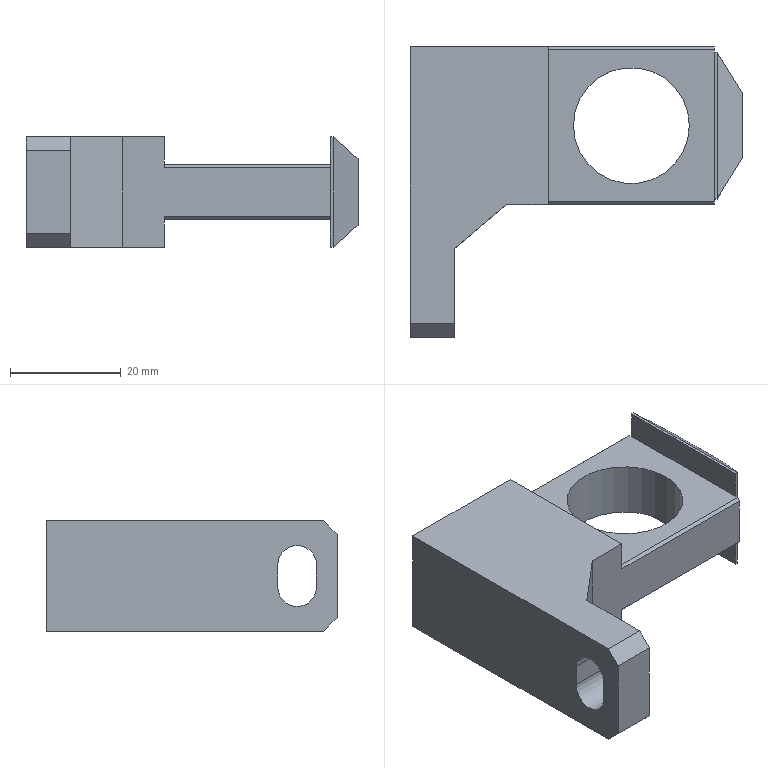Part | STEP file | HI_BC4000 Br | 1 solid | 44 faces | box 60 x 52.5 x 20 mm | volume 24751 mm3 | plane 35 | cylinder 9 | commonest cylinder face diameters 7 x3 6 x2 8 x2 20.955 x2
STEP:
#1=CARTESIAN_POINT('',(-32.,-31.,5.5));
#2=VERTEX_POINT('',#1);
#3=CARTESIAN_POINT('',(-32.,-27.5,2.));
#4=VERTEX_POINT('',#3);
#5=CARTESIAN_POINT('',(-32.,-31.,2.));
#6=DIRECTION('',(-1.,0.,0.));
#7=DIRECTION('',(0.,0.,1.));
#8=AXIS2_PLACEMENT_3D('',#5,#6,#7);
#9=CIRCLE('',#8,3.5);
#10=EDGE_CURVE('',#2,#4,#9,.T.);
#11=ORIENTED_EDGE('',*,*,#10,.F.);
#12=CARTESIAN_POINT('',(-40.,-31.,5.5));
#13=VERTEX_POINT('',#12);
#14=CARTESIAN_POINT('',(-40.,-31.,5.5));
#15=DIRECTION('',(-1.,0.,0.));
#16=VECTOR('',#15,1000.);
#17=LINE('',#14,#16);
#18=EDGE_CURVE('',#2,#13,#17,.T.);
#19=ORIENTED_EDGE('',*,*,#18,.T.);
#20=CARTESIAN_POINT('',(-40.,-27.5,2.));
#21=VERTEX_POINT('',#20);
#22=CARTESIAN_POINT('',(-40.,-31.,2.));
#23=DIRECTION('',(-1.,0.,0.));
#24=DIRECTION('',(0.,0.,1.));
#25=AXIS2_PLACEMENT_3D('',#22,#23,#24);
#26=CIRCLE('',#25,3.5);
#27=EDGE_CURVE('',#13,#21,#26,.T.);
#28=ORIENTED_EDGE('',*,*,#27,.T.);
#29=CARTESIAN_POINT('',(-40.,-27.5,2.));
#30=DIRECTION('',(1.,0.,0.));
#31=VECTOR('',#30,1000.);
#32=LINE('',#29,#31);
#33=EDGE_CURVE('',#21,#4,#32,.T.);
#34=ORIENTED_EDGE('',*,*,#33,.T.);
#35=EDGE_LOOP('',(#11,#19,#28,#34));
#36=FACE_OUTER_BOUND('',#35,.T.);
#37=CARTESIAN_POINT('',(-40.,-31.,2.));
#38=DIRECTION('',(-1.,0.,0.));
#39=DIRECTION('',(0.,0.,1.));
#40=AXIS2_PLACEMENT_3D('',#37,#38,#39);
#41=CYLINDRICAL_SURFACE('',#40,3.5);
#42=ADVANCED_FACE('',(#36),#41,.F.);
#43=CARTESIAN_POINT('',(10.477,0.,-5.));
#44=VERTEX_POINT('',#43);
#45=CARTESIAN_POINT('',(-10.477,0.,-5.));
#46=VERTEX_POINT('',#45);
#47=CARTESIAN_POINT('',(0.,0.,-5.));
#48=DIRECTION('',(0.,0.,-1.));
#49=DIRECTION('',(1.,0.,0.));
#50=AXIS2_PLACEMENT_3D('',#47,#48,#49);
#51=CIRCLE('',#50,10.477);
#52=EDGE_CURVE('',#44,#46,#51,.T.);
#53=ORIENTED_EDGE('',*,*,#52,.T.);
#54=CARTESIAN_POINT('',(-10.477,0.,5.));
#55=VERTEX_POINT('',#54);
#56=CARTESIAN_POINT('',(-10.477,0.,5.));
#57=DIRECTION('',(0.,0.,1.));
#58=VECTOR('',#57,1000.);
#59=LINE('',#56,#58);
#60=EDGE_CURVE('',#46,#55,#59,.T.);
#61=ORIENTED_EDGE('',*,*,#60,.T.);
#62=CARTESIAN_POINT('',(10.477,0.,5.));
#63=VERTEX_POINT('',#62);
#64=CARTESIAN_POINT('',(0.,0.,5.));
#65=DIRECTION('',(0.,0.,1.));
#66=DIRECTION('',(1.,0.,0.));
#67=AXIS2_PLACEMENT_3D('',#64,#65,#66);
#68=CIRCLE('',#67,10.477);
#69=EDGE_CURVE('',#55,#63,#68,.T.);
#70=ORIENTED_EDGE('',*,*,#69,.T.);
#71=CARTESIAN_POINT('',(10.477,0.,5.));
#72=DIRECTION('',(0.,0.,1.));
#73=VECTOR('',#72,1000.);
#74=LINE('',#71,#73);
#75=EDGE_CURVE('',#44,#63,#74,.T.);
#76=ORIENTED_EDGE('',*,*,#75,.F.);
#77=EDGE_LOOP('',(#53,#61,#70,#76));
#78=FACE_OUTER_BOUND('',#77,.T.);
#79=CARTESIAN_POINT('',(0.,0.,5.));
#80=DIRECTION('',(0.,0.,1.));
#81=DIRECTION('',(1.,0.,0.));
#82=AXIS2_PLACEMENT_3D('',#79,#80,#81);
#83=CYLINDRICAL_SURFACE('',#82,10.477);
#84=ADVANCED_FACE('',(#78),#83,.F.);
#85=CARTESIAN_POINT('',(20.,0.,4.));
#86=VERTEX_POINT('',#85);
#87=CARTESIAN_POINT('',(20.,0.,-4.));
#88=VERTEX_POINT('',#87);
#89=CARTESIAN_POINT('',(20.,0.,0.));
#90=DIRECTION('',(1.,0.,0.));
#91=DIRECTION('',(0.,0.,1.));
#92=AXIS2_PLACEMENT_3D('',#89,#90,#91);
#93=CIRCLE('',#92,4.);
#94=EDGE_CURVE('',#86,#88,#93,.T.);
#95=ORIENTED_EDGE('',*,*,#94,.T.);
#96=CARTESIAN_POINT('',(17.,0.,-4.));
#97=VERTEX_POINT('',#96);
#98=CARTESIAN_POINT('',(20.,0.,-4.));
#99=DIRECTION('',(-1.,0.,0.));
#100=VECTOR('',#99,1000.);
#101=LINE('',#98,#100);
#102=EDGE_CURVE('',#88,#97,#101,.T.);
#103=ORIENTED_EDGE('',*,*,#102,.T.);
#104=CARTESIAN_POINT('',(17.,0.,4.));
#105=VERTEX_POINT('',#104);
#106=CARTESIAN_POINT('',(17.,0.,0.));
#107=DIRECTION('',(1.,0.,0.));
#108=DIRECTION('',(0.,0.,1.));
#109=AXIS2_PLACEMENT_3D('',#106,#107,#108);
#110=CIRCLE('',#109,4.);
#111=EDGE_CURVE('',#105,#97,#110,.T.);
#112=ORIENTED_EDGE('',*,*,#111,.F.);
#113=CARTESIAN_POINT('',(20.,0.,4.));
#114=DIRECTION('',(-1.,0.,0.));
#115=VECTOR('',#114,1000.);
#116=LINE('',#113,#115);
#117=EDGE_CURVE('',#86,#105,#116,.T.);
#118=ORIENTED_EDGE('',*,*,#117,.F.);
#119=EDGE_LOOP('',(#95,#103,#112,#118));
#120=FACE_OUTER_BOUND('',#119,.T.);
#121=CARTESIAN_POINT('',(20.,0.,0.));
#122=DIRECTION('',(-1.,0.,0.));
#123=DIRECTION('',(0.,0.,1.));
#124=AXIS2_PLACEMENT_3D('',#121,#122,#123);
#125=CYLINDRICAL_SURFACE('',#124,4.);
#126=ADVANCED_FACE('',(#120),#125,.F.);
#127=CARTESIAN_POINT('',(17.,0.,-3.));
#128=VERTEX_POINT('',#127);
#129=CARTESIAN_POINT('',(17.,0.,3.));
#130=VERTEX_POINT('',#129);
#131=CARTESIAN_POINT('',(17.,0.,0.));
#132=DIRECTION('',(-1.,0.,0.));
#133=DIRECTION('',(0.,0.,1.));
#134=AXIS2_PLACEMENT_3D('',#131,#132,#133);
#135=CIRCLE('',#134,3.);
#136=EDGE_CURVE('',#128,#130,#135,.T.);
#137=ORIENTED_EDGE('',*,*,#136,.F.);
#138=CARTESIAN_POINT('',(12.,0.,-3.));
#139=VERTEX_POINT('',#138);
#140=CARTESIAN_POINT('',(20.,0.,-3.));
#141=DIRECTION('',(-1.,0.,0.));
#142=VECTOR('',#141,1000.);
#143=LINE('',#140,#142);
#144=EDGE_CURVE('',#128,#139,#143,.T.);
#145=ORIENTED_EDGE('',*,*,#144,.T.);
#146=CARTESIAN_POINT('',(12.,0.,3.));
#147=VERTEX_POINT('',#146);
#148=CARTESIAN_POINT('',(12.,0.,0.));
#149=DIRECTION('',(1.,0.,0.));
#150=DIRECTION('',(0.,0.,1.));
#151=AXIS2_PLACEMENT_3D('',#148,#149,#150);
#152=CIRCLE('',#151,3.);
#153=EDGE_CURVE('',#147,#139,#152,.T.);
#154=ORIENTED_EDGE('',*,*,#153,.F.);
#155=CARTESIAN_POINT('',(20.,0.,3.));
#156=DIRECTION('',(-1.,0.,0.));
#157=VECTOR('',#156,1000.);
#158=LINE('',#155,#157);
#159=EDGE_CURVE('',#130,#147,#158,.T.);
#160=ORIENTED_EDGE('',*,*,#159,.F.);
#161=EDGE_LOOP('',(#137,#145,#154,#160));
#162=FACE_OUTER_BOUND('',#161,.T.);
#163=CARTESIAN_POINT('',(20.,0.,0.));
#164=DIRECTION('',(-1.,0.,0.));
#165=DIRECTION('',(0.,0.,1.));
#166=AXIS2_PLACEMENT_3D('',#163,#164,#165);
#167=CYLINDRICAL_SURFACE('',#166,3.);
#168=ADVANCED_FACE('',(#162),#167,.F.);
#169=CARTESIAN_POINT('',(-40.,-35.75,10.));
#170=VERTEX_POINT('',#169);
#171=CARTESIAN_POINT('',(-40.,-38.25,7.5));
#172=VERTEX_POINT('',#171);
#173=CARTESIAN_POINT('',(-40.,-35.75,10.));
#174=DIRECTION('',(0.,-0.7071,-0.7071));
#175=VECTOR('',#174,1000.);
#176=LINE('',#173,#175);
#177=EDGE_CURVE('',#170,#172,#176,.T.);
#178=ORIENTED_EDGE('',*,*,#177,.F.);
#179=CARTESIAN_POINT('',(-40.,14.25,10.));
#180=VERTEX_POINT('',#179);
#181=CARTESIAN_POINT('',(-40.,14.25,10.));
#182=DIRECTION('',(0.,-1.,0.));
#183=VECTOR('',#182,1000.);
#184=LINE('',#181,#183);
#185=EDGE_CURVE('',#180,#170,#184,.T.);
#186=ORIENTED_EDGE('',*,*,#185,.F.);
#187=CARTESIAN_POINT('',(-40.,14.25,-10.));
#188=VERTEX_POINT('',#187);
#189=CARTESIAN_POINT('',(-40.,14.25,10.));
#190=DIRECTION('',(0.,0.,1.));
#191=VECTOR('',#190,1000.);
#192=LINE('',#189,#191);
#193=EDGE_CURVE('',#188,#180,#192,.T.);
#194=ORIENTED_EDGE('',*,*,#193,.F.);
#195=CARTESIAN_POINT('',(-40.,-35.75,-10.));
#196=VERTEX_POINT('',#195);
#197=CARTESIAN_POINT('',(-40.,14.25,-10.));
#198=DIRECTION('',(0.,1.,0.));
#199=VECTOR('',#198,1000.);
#200=LINE('',#197,#199);
#201=EDGE_CURVE('',#196,#188,#200,.T.);
#202=ORIENTED_EDGE('',*,*,#201,.F.);
#203=CARTESIAN_POINT('',(-40.,-38.25,-7.5));
#204=VERTEX_POINT('',#203);
#205=CARTESIAN_POINT('',(-40.,-38.25,-7.5));
#206=DIRECTION('',(0.,0.7071,-0.7071));
#207=VECTOR('',#206,1000.);
#208=LINE('',#205,#207);
#209=EDGE_CURVE('',#204,#196,#208,.T.);
#210=ORIENTED_EDGE('',*,*,#209,.F.);
#211=CARTESIAN_POINT('',(-40.,-38.25,10.));
#212=DIRECTION('',(0.,0.,-1.));
#213=VECTOR('',#212,1000.);
#214=LINE('',#211,#213);
#215=EDGE_CURVE('',#172,#204,#214,.T.);
#216=ORIENTED_EDGE('',*,*,#215,.F.);
#217=EDGE_LOOP('',(#178,#186,#194,#202,#210,#216));
#218=FACE_OUTER_BOUND('',#217,.T.);
#219=CARTESIAN_POINT('',(-40.,-27.5,-2.));
#220=VERTEX_POINT('',#219);
#221=CARTESIAN_POINT('',(-40.,-27.5,10.));
#222=DIRECTION('',(0.,0.,-1.));
#223=VECTOR('',#222,1000.);
#224=LINE('',#221,#223);
#225=EDGE_CURVE('',#21,#220,#224,.T.);
#226=ORIENTED_EDGE('',*,*,#225,.F.);
#227=ORIENTED_EDGE('',*,*,#27,.F.);
#228=CARTESIAN_POINT('',(-40.,-34.5,2.));
#229=VERTEX_POINT('',#228);
#230=CARTESIAN_POINT('',(-40.,-31.,2.));
#231=DIRECTION('',(-1.,0.,0.));
#232=DIRECTION('',(0.,0.,1.));
#233=AXIS2_PLACEMENT_3D('',#230,#231,#232);
#234=CIRCLE('',#233,3.5);
#235=EDGE_CURVE('',#229,#13,#234,.T.);
#236=ORIENTED_EDGE('',*,*,#235,.F.);
#237=CARTESIAN_POINT('',(-40.,-34.5,-2.));
#238=VERTEX_POINT('',#237);
#239=CARTESIAN_POINT('',(-40.,-34.5,10.));
#240=DIRECTION('',(0.,0.,1.));
#241=VECTOR('',#240,1000.);
#242=LINE('',#239,#241);
#243=EDGE_CURVE('',#238,#229,#242,.T.);
#244=ORIENTED_EDGE('',*,*,#243,.F.);
#245=CARTESIAN_POINT('',(-40.,-31.,-2.));
#246=DIRECTION('',(-1.,0.,0.));
#247=DIRECTION('',(0.,0.,1.));
#248=AXIS2_PLACEMENT_3D('',#245,#246,#247);
#249=CIRCLE('',#248,3.5);
#250=EDGE_CURVE('',#220,#238,#249,.T.);
#251=ORIENTED_EDGE('',*,*,#250,.F.);
#252=EDGE_LOOP('',(#226,#227,#236,#244,#251));
#253=FACE_BOUND('',#252,.T.);
#254=CARTESIAN_POINT('',(-40.,14.25,10.));
#255=DIRECTION('',(1.,0.,0.));
#256=DIRECTION('',(0.,0.,-1.));
#257=AXIS2_PLACEMENT_3D('',#254,#255,#256);
#258=PLANE('',#257);
#259=ADVANCED_FACE('',(#218,#253),#258,.F.);
#260=CARTESIAN_POINT('',(-32.,-38.25,7.5));
#261=VERTEX_POINT('',#260);
#262=CARTESIAN_POINT('',(-40.,-38.25,7.5));
#263=DIRECTION('',(1.,0.,0.));
#264=VECTOR('',#263,1000.);
#265=LINE('',#262,#264);
#266=EDGE_CURVE('',#172,#261,#265,.T.);
#267=ORIENTED_EDGE('',*,*,#266,.F.);
#268=ORIENTED_EDGE('',*,*,#215,.T.);
#269=CARTESIAN_POINT('',(-32.,-38.25,-7.5));
#270=VERTEX_POINT('',#269);
#271=CARTESIAN_POINT('',(-40.,-38.25,-7.5));
#272=DIRECTION('',(-1.,0.,0.));
#273=VECTOR('',#272,1000.);
#274=LINE('',#271,#273);
#275=EDGE_CURVE('',#270,#204,#274,.T.);
#276=ORIENTED_EDGE('',*,*,#275,.F.);
#277=CARTESIAN_POINT('',(-32.,-38.25,10.));
#278=DIRECTION('',(0.,0.,-1.));
#279=VECTOR('',#278,1000.);
#280=LINE('',#277,#279);
#281=EDGE_CURVE('',#261,#270,#280,.T.);
#282=ORIENTED_EDGE('',*,*,#281,.F.);
#283=EDGE_LOOP('',(#267,#268,#276,#282));
#284=FACE_OUTER_BOUND('',#283,.T.);
#285=CARTESIAN_POINT('',(-40.,-38.25,10.));
#286=DIRECTION('',(0.,1.,0.));
#287=DIRECTION('',(0.,0.,1.));
#288=AXIS2_PLACEMENT_3D('',#285,#286,#287);
#289=PLANE('',#288);
#290=ADVANCED_FACE('',(#284),#289,.F.);
#291=ORIENTED_EDGE('',*,*,#177,.T.);
#292=ORIENTED_EDGE('',*,*,#266,.T.);
#293=CARTESIAN_POINT('',(-32.,-35.75,10.));
#294=VERTEX_POINT('',#293);
#295=CARTESIAN_POINT('',(-32.,-38.25,7.5));
#296=DIRECTION('',(0.,-0.7071,-0.7071));
#297=VECTOR('',#296,1000.);
#298=LINE('',#295,#297);
#299=EDGE_CURVE('',#294,#261,#298,.T.);
#300=ORIENTED_EDGE('',*,*,#299,.F.);
#301=CARTESIAN_POINT('',(-40.,-35.75,10.));
#302=DIRECTION('',(1.,0.,0.));
#303=VECTOR('',#302,1000.);
#304=LINE('',#301,#303);
#305=EDGE_CURVE('',#170,#294,#304,.T.);
#306=ORIENTED_EDGE('',*,*,#305,.F.);
#307=EDGE_LOOP('',(#291,#292,#300,#306));
#308=FACE_OUTER_BOUND('',#307,.T.);
#309=CARTESIAN_POINT('',(-40.,-38.25,7.5));
#310=DIRECTION('',(0.,0.7071,-0.7071));
#311=DIRECTION('',(0.,0.7071,0.7071));
#312=AXIS2_PLACEMENT_3D('',#309,#310,#311);
#313=PLANE('',#312);
#314=ADVANCED_FACE('',(#308),#313,.F.);
#315=CARTESIAN_POINT('',(-15.,14.25,10.));
#316=VERTEX_POINT('',#315);
#317=CARTESIAN_POINT('',(0.,14.25,10.));
#318=DIRECTION('',(-1.,0.,0.));
#319=VECTOR('',#318,1000.);
#320=LINE('',#317,#319);
#321=EDGE_CURVE('',#316,#180,#320,.T.);
#322=ORIENTED_EDGE('',*,*,#321,.T.);
#323=ORIENTED_EDGE('',*,*,#185,.T.);
#324=ORIENTED_EDGE('',*,*,#305,.T.);
#325=CARTESIAN_POINT('',(-32.,-22.25,10.));
#326=VERTEX_POINT('',#325);
#327=CARTESIAN_POINT('',(-32.,0.,10.));
#328=DIRECTION('',(0.,1.,0.));
#329=VECTOR('',#328,1000.);
#330=LINE('',#327,#329);
#331=EDGE_CURVE('',#294,#326,#330,.T.);
#332=ORIENTED_EDGE('',*,*,#331,.T.);
#333=CARTESIAN_POINT('',(-22.569,-14.25,10.));
#334=VERTEX_POINT('',#333);
#335=CARTESIAN_POINT('',(-32.,-22.25,10.));
#336=DIRECTION('',(0.7626,0.6469,0.));
#337=VECTOR('',#336,1000.);
#338=LINE('',#335,#337);
#339=EDGE_CURVE('',#326,#334,#338,.T.);
#340=ORIENTED_EDGE('',*,*,#339,.T.);
#341=CARTESIAN_POINT('',(-15.,-14.25,10.));
#342=VERTEX_POINT('',#341);
#343=CARTESIAN_POINT('',(0.,-14.25,10.));
#344=DIRECTION('',(1.,0.,0.));
#345=VECTOR('',#344,1000.);
#346=LINE('',#343,#345);
#347=EDGE_CURVE('',#334,#342,#346,.T.);
#348=ORIENTED_EDGE('',*,*,#347,.T.);
#349=CARTESIAN_POINT('',(-15.,0.,10.));
#350=DIRECTION('',(0.,1.,0.));
#351=VECTOR('',#350,1000.);
#352=LINE('',#349,#351);
#353=EDGE_CURVE('',#342,#316,#352,.T.);
#354=ORIENTED_EDGE('',*,*,#353,.T.);
#355=EDGE_LOOP('',(#322,#323,#324,#332,#340,#348,#354));
#356=FACE_OUTER_BOUND('',#355,.T.);
#357=CARTESIAN_POINT('',(0.,0.,10.));
#358=DIRECTION('',(0.,0.,1.));
#359=DIRECTION('',(1.,0.,0.));
#360=AXIS2_PLACEMENT_3D('',#357,#358,#359);
#361=PLANE('',#360);
#362=ADVANCED_FACE('',(#356),#361,.T.);
#363=CARTESIAN_POINT('',(-15.,14.25,-10.));
#364=VERTEX_POINT('',#363);
#365=CARTESIAN_POINT('',(-15.,14.25,-4.5));
#366=VERTEX_POINT('',#365);
#367=CARTESIAN_POINT('',(-15.,14.25,-4.5));
#368=DIRECTION('',(0.,0.,1.));
#369=VECTOR('',#368,1000.);
#370=LINE('',#367,#369);
#371=EDGE_CURVE('',#364,#366,#370,.T.);
#372=ORIENTED_EDGE('',*,*,#371,.F.);
#373=CARTESIAN_POINT('',(15.,14.25,-10.));
#374=DIRECTION('',(1.,0.,0.));
#375=VECTOR('',#374,1000.);
#376=LINE('',#373,#375);
#377=EDGE_CURVE('',#188,#364,#376,.T.);
#378=ORIENTED_EDGE('',*,*,#377,.F.);
#379=ORIENTED_EDGE('',*,*,#193,.T.);
#380=ORIENTED_EDGE('',*,*,#321,.F.);
#381=CARTESIAN_POINT('',(-15.,14.25,4.5));
#382=VERTEX_POINT('',#381);
#383=CARTESIAN_POINT('',(-15.,14.25,-4.5));
#384=DIRECTION('',(0.,0.,1.));
#385=VECTOR('',#384,1000.);
#386=LINE('',#383,#385);
#387=EDGE_CURVE('',#382,#316,#386,.T.);
#388=ORIENTED_EDGE('',*,*,#387,.F.);
#389=CARTESIAN_POINT('',(15.,14.25,4.5));
#390=VERTEX_POINT('',#389);
#391=CARTESIAN_POINT('',(15.,14.25,4.5));
#392=DIRECTION('',(-1.,0.,0.));
#393=VECTOR('',#392,1000.);
#394=LINE('',#391,#393);
#395=EDGE_CURVE('',#390,#382,#394,.T.);
#396=ORIENTED_EDGE('',*,*,#395,.F.);
#397=CARTESIAN_POINT('',(15.,14.25,-4.5));
#398=VERTEX_POINT('',#397);
#399=CARTESIAN_POINT('',(15.,14.25,-4.5));
#400=DIRECTION('',(0.,0.,1.));
#401=VECTOR('',#400,1000.);
#402=LINE('',#399,#401);
#403=EDGE_CURVE('',#398,#390,#402,.T.);
#404=ORIENTED_EDGE('',*,*,#403,.F.);
#405=CARTESIAN_POINT('',(15.,14.25,-4.5));
#406=DIRECTION('',(1.,0.,0.));
#407=VECTOR('',#406,1000.);
#408=LINE('',#405,#407);
#409=EDGE_CURVE('',#366,#398,#408,.T.);
#410=ORIENTED_EDGE('',*,*,#409,.F.);
#411=EDGE_LOOP('',(#372,#378,#379,#380,#388,#396,#404,#410));
#412=FACE_OUTER_BOUND('',#411,.T.);
#413=CARTESIAN_POINT('',(15.,14.25,-4.5));
#414=DIRECTION('',(0.,-1.,0.));
#415=DIRECTION('',(0.,0.,-1.));
#416=AXIS2_PLACEMENT_3D('',#413,#414,#415);
#417=PLANE('',#416);
#418=ADVANCED_FACE('',(#412),#417,.F.);
#419=CARTESIAN_POINT('',(-32.,-35.75,-10.));
#420=VERTEX_POINT('',#419);
#421=CARTESIAN_POINT('',(0.,-35.75,-10.));
#422=DIRECTION('',(1.,0.,0.));
#423=VECTOR('',#422,1000.);
#424=LINE('',#421,#423);
#425=EDGE_CURVE('',#196,#420,#424,.T.);
#426=ORIENTED_EDGE('',*,*,#425,.F.);
#427=ORIENTED_EDGE('',*,*,#201,.T.);
#428=ORIENTED_EDGE('',*,*,#377,.T.);
#429=CARTESIAN_POINT('',(-15.,-14.25,-10.));
#430=VERTEX_POINT('',#429);
#431=CARTESIAN_POINT('',(-15.,0.,-10.));
#432=DIRECTION('',(0.,1.,0.));
#433=VECTOR('',#432,1000.);
#434=LINE('',#431,#433);
#435=EDGE_CURVE('',#430,#364,#434,.T.);
#436=ORIENTED_EDGE('',*,*,#435,.F.);
#437=CARTESIAN_POINT('',(-22.569,-14.25,-10.));
#438=VERTEX_POINT('',#437);
#439=CARTESIAN_POINT('',(0.,-14.25,-10.));
#440=DIRECTION('',(1.,0.,0.));
#441=VECTOR('',#440,1000.);
#442=LINE('',#439,#441);
#443=EDGE_CURVE('',#438,#430,#442,.T.);
#444=ORIENTED_EDGE('',*,*,#443,.F.);
#445=CARTESIAN_POINT('',(-32.,-22.25,-10.));
#446=VERTEX_POINT('',#445);
#447=CARTESIAN_POINT('',(-32.,-22.25,-10.));
#448=DIRECTION('',(0.7626,0.6469,0.));
#449=VECTOR('',#448,1000.);
#450=LINE('',#447,#449);
#451=EDGE_CURVE('',#446,#438,#450,.T.);
#452=ORIENTED_EDGE('',*,*,#451,.F.);
#453=CARTESIAN_POINT('',(-32.,0.,-10.));
#454=DIRECTION('',(0.,1.,0.));
#455=VECTOR('',#454,1000.);
#456=LINE('',#453,#455);
#457=EDGE_CURVE('',#420,#446,#456,.T.);
#458=ORIENTED_EDGE('',*,*,#457,.F.);
#459=EDGE_LOOP('',(#426,#427,#428,#436,#444,#452,#458));
#460=FACE_OUTER_BOUND('',#459,.T.);
#461=CARTESIAN_POINT('',(0.,0.,-10.));
#462=DIRECTION('',(0.,0.,1.));
#463=DIRECTION('',(1.,0.,0.));
#464=AXIS2_PLACEMENT_3D('',#461,#462,#463);
#465=PLANE('',#464);
#466=ADVANCED_FACE('',(#460),#465,.F.);
#467=ORIENTED_EDGE('',*,*,#209,.T.);
#468=ORIENTED_EDGE('',*,*,#425,.T.);
#469=CARTESIAN_POINT('',(-32.,-35.75,-10.));
#470=DIRECTION('',(0.,0.7071,-0.7071));
#471=VECTOR('',#470,1000.);
#472=LINE('',#469,#471);
#473=EDGE_CURVE('',#270,#420,#472,.T.);
#474=ORIENTED_EDGE('',*,*,#473,.F.);
#475=ORIENTED_EDGE('',*,*,#275,.T.);
#476=EDGE_LOOP('',(#467,#468,#474,#475));
#477=FACE_OUTER_BOUND('',#476,.T.);
#478=CARTESIAN_POINT('',(-40.,-35.75,-10.));
#479=DIRECTION('',(0.,0.7071,0.7071));
#480=DIRECTION('',(0.,-0.7071,0.7071));
#481=AXIS2_PLACEMENT_3D('',#478,#479,#480);
#482=PLANE('',#481);
#483=ADVANCED_FACE('',(#477),#482,.F.);
#484=ORIENTED_EDGE('',*,*,#250,.T.);
#485=CARTESIAN_POINT('',(-32.,-34.5,-2.));
#486=VERTEX_POINT('',#485);
#487=CARTESIAN_POINT('',(-40.,-34.5,-2.));
#488=DIRECTION('',(-1.,0.,0.));
#489=VECTOR('',#488,1000.);
#490=LINE('',#487,#489);
#491=EDGE_CURVE('',#486,#238,#490,.T.);
#492=ORIENTED_EDGE('',*,*,#491,.F.);
#493=CARTESIAN_POINT('',(-32.,-27.5,-2.));
#494=VERTEX_POINT('',#493);
#495=CARTESIAN_POINT('',(-32.,-31.,-2.));
#496=DIRECTION('',(-1.,0.,0.));
#497=DIRECTION('',(0.,0.,1.));
#498=AXIS2_PLACEMENT_3D('',#495,#496,#497);
#499=CIRCLE('',#498,3.5);
#500=EDGE_CURVE('',#494,#486,#499,.T.);
#501=ORIENTED_EDGE('',*,*,#500,.F.);
#502=CARTESIAN_POINT('',(-40.,-27.5,-2.));
#503=DIRECTION('',(1.,0.,0.));
#504=VECTOR('',#503,1000.);
#505=LINE('',#502,#504);
#506=EDGE_CURVE('',#220,#494,#505,.T.);
#507=ORIENTED_EDGE('',*,*,#506,.F.);
#508=EDGE_LOOP('',(#484,#492,#501,#507));
#509=FACE_OUTER_BOUND('',#508,.T.);
#510=CARTESIAN_POINT('',(-40.,-31.,-2.));
#511=DIRECTION('',(-1.,0.,0.));
#512=DIRECTION('',(0.,0.,1.));
#513=AXIS2_PLACEMENT_3D('',#510,#511,#512);
#514=CYLINDRICAL_SURFACE('',#513,3.5);
#515=ADVANCED_FACE('',(#509),#514,.F.);
#516=ORIENTED_EDGE('',*,*,#225,.T.);
#517=ORIENTED_EDGE('',*,*,#506,.T.);
#518=CARTESIAN_POINT('',(-32.,-27.5,-2.));
#519=DIRECTION('',(0.,0.,-1.));
#520=VECTOR('',#519,1000.);
#521=LINE('',#518,#520);
#522=EDGE_CURVE('',#4,#494,#521,.T.);
#523=ORIENTED_EDGE('',*,*,#522,.F.);
#524=ORIENTED_EDGE('',*,*,#33,.F.);
#525=EDGE_LOOP('',(#516,#517,#523,#524));
#526=FACE_OUTER_BOUND('',#525,.T.);
#527=CARTESIAN_POINT('',(-40.,-27.5,-2.));
#528=DIRECTION('',(0.,1.,0.));
#529=DIRECTION('',(0.,0.,1.));
#530=AXIS2_PLACEMENT_3D('',#527,#528,#529);
#531=PLANE('',#530);
#532=ADVANCED_FACE('',(#526),#531,.F.);
#533=ORIENTED_EDGE('',*,*,#18,.F.);
#534=CARTESIAN_POINT('',(-32.,-34.5,2.));
#535=VERTEX_POINT('',#534);
#536=CARTESIAN_POINT('',(-32.,-31.,2.));
#537=DIRECTION('',(-1.,0.,0.));
#538=DIRECTION('',(0.,0.,1.));
#539=AXIS2_PLACEMENT_3D('',#536,#537,#538);
#540=CIRCLE('',#539,3.5);
#541=EDGE_CURVE('',#535,#2,#540,.T.);
#542=ORIENTED_EDGE('',*,*,#541,.F.);
#543=CARTESIAN_POINT('',(-40.,-34.5,2.));
#544=DIRECTION('',(1.,0.,0.));
#545=VECTOR('',#544,1000.);
#546=LINE('',#543,#545);
#547=EDGE_CURVE('',#229,#535,#546,.T.);
#548=ORIENTED_EDGE('',*,*,#547,.F.);
#549=ORIENTED_EDGE('',*,*,#235,.T.);
#550=EDGE_LOOP('',(#533,#542,#548,#549));
#551=FACE_OUTER_BOUND('',#550,.T.);
#552=CARTESIAN_POINT('',(-40.,-31.,2.));
#553=DIRECTION('',(-1.,0.,0.));
#554=DIRECTION('',(0.,0.,1.));
#555=AXIS2_PLACEMENT_3D('',#552,#553,#554);
#556=CYLINDRICAL_SURFACE('',#555,3.5);
#557=ADVANCED_FACE('',(#551),#556,.F.);
#558=ORIENTED_EDGE('',*,*,#243,.T.);
#559=ORIENTED_EDGE('',*,*,#547,.T.);
#560=CARTESIAN_POINT('',(-32.,-34.5,2.));
#561=DIRECTION('',(0.,0.,1.));
#562=VECTOR('',#561,1000.);
#563=LINE('',#560,#562);
#564=EDGE_CURVE('',#486,#535,#563,.T.);
#565=ORIENTED_EDGE('',*,*,#564,.F.);
#566=ORIENTED_EDGE('',*,*,#491,.T.);
#567=EDGE_LOOP('',(#558,#559,#565,#566));
#568=FACE_OUTER_BOUND('',#567,.T.);
#569=CARTESIAN_POINT('',(-40.,-34.5,2.));
#570=DIRECTION('',(0.,-1.,0.));
#571=DIRECTION('',(0.,0.,-1.));
#572=AXIS2_PLACEMENT_3D('',#569,#570,#571);
#573=PLANE('',#572);
#574=ADVANCED_FACE('',(#568),#573,.F.);
#575=ORIENTED_EDGE('',*,*,#299,.T.);
#576=ORIENTED_EDGE('',*,*,#281,.T.);
#577=ORIENTED_EDGE('',*,*,#473,.T.);
#578=ORIENTED_EDGE('',*,*,#457,.T.);
#579=CARTESIAN_POINT('',(-32.,-22.25,10.));
#580=DIRECTION('',(0.,0.,-1.));
#581=VECTOR('',#580,1000.);
#582=LINE('',#579,#581);
#583=EDGE_CURVE('',#326,#446,#582,.T.);
#584=ORIENTED_EDGE('',*,*,#583,.F.);
#585=ORIENTED_EDGE('',*,*,#331,.F.);
#586=EDGE_LOOP('',(#575,#576,#577,#578,#584,#585));
#587=FACE_OUTER_BOUND('',#586,.T.);
#588=ORIENTED_EDGE('',*,*,#522,.T.);
#589=ORIENTED_EDGE('',*,*,#500,.T.);
#590=ORIENTED_EDGE('',*,*,#564,.T.);
#591=ORIENTED_EDGE('',*,*,#541,.T.);
#592=ORIENTED_EDGE('',*,*,#10,.T.);
#593=EDGE_LOOP('',(#588,#589,#590,#591,#592));
#594=FACE_BOUND('',#593,.T.);
#595=CARTESIAN_POINT('',(-32.,-38.25,10.));
#596=DIRECTION('',(-1.,0.,0.));
#597=DIRECTION('',(0.,0.,1.));
#598=AXIS2_PLACEMENT_3D('',#595,#596,#597);
#599=PLANE('',#598);
#600=ADVANCED_FACE('',(#587,#594),#599,.F.);
#601=ORIENTED_EDGE('',*,*,#387,.T.);
#602=ORIENTED_EDGE('',*,*,#353,.F.);
#603=CARTESIAN_POINT('',(-15.,-14.25,4.5));
#604=VERTEX_POINT('',#603);
#605=CARTESIAN_POINT('',(-15.,-14.25,10.));
#606=DIRECTION('',(0.,0.,1.));
#607=VECTOR('',#606,1000.);
#608=LINE('',#605,#607);
#609=EDGE_CURVE('',#604,#342,#608,.T.);
#610=ORIENTED_EDGE('',*,*,#609,.F.);
#611=CARTESIAN_POINT('',(-15.,-13.75,5.));
#612=VERTEX_POINT('',#611);
#613=CARTESIAN_POINT('',(-15.,-13.75,5.));
#614=DIRECTION('',(0.,0.7071,0.7071));
#615=VECTOR('',#614,1000.);
#616=LINE('',#613,#615);
#617=EDGE_CURVE('',#604,#612,#616,.T.);
#618=ORIENTED_EDGE('',*,*,#617,.T.);
#619=CARTESIAN_POINT('',(-15.,13.75,5.));
#620=VERTEX_POINT('',#619);
#621=CARTESIAN_POINT('',(-15.,-14.25,5.));
#622=DIRECTION('',(0.,-1.,0.));
#623=VECTOR('',#622,1000.);
#624=LINE('',#621,#623);
#625=EDGE_CURVE('',#620,#612,#624,.T.);
#626=ORIENTED_EDGE('',*,*,#625,.F.);
#627=CARTESIAN_POINT('',(-15.,14.25,4.5));
#628=DIRECTION('',(0.,-0.7071,0.7071));
#629=VECTOR('',#628,1000.);
#630=LINE('',#627,#629);
#631=EDGE_CURVE('',#382,#620,#630,.T.);
#632=ORIENTED_EDGE('',*,*,#631,.F.);
#633=EDGE_LOOP('',(#601,#602,#610,#618,#626,#632));
#634=FACE_OUTER_BOUND('',#633,.T.);
#635=CARTESIAN_POINT('',(-15.,-14.25,10.));
#636=DIRECTION('',(-1.,0.,0.));
#637=DIRECTION('',(0.,0.,1.));
#638=AXIS2_PLACEMENT_3D('',#635,#636,#637);
#639=PLANE('',#638);
#640=ADVANCED_FACE('',(#634),#639,.F.);
#641=ORIENTED_EDGE('',*,*,#609,.T.);
#642=ORIENTED_EDGE('',*,*,#347,.F.);
#643=CARTESIAN_POINT('',(-22.569,-14.25,4.5));
#644=DIRECTION('',(0.,0.,1.));
#645=VECTOR('',#644,1000.);
#646=LINE('',#643,#645);
#647=EDGE_CURVE('',#438,#334,#646,.T.);
#648=ORIENTED_EDGE('',*,*,#647,.F.);
#649=ORIENTED_EDGE('',*,*,#443,.T.);
#650=CARTESIAN_POINT('',(-15.,-14.25,-4.5));
#651=VERTEX_POINT('',#650);
#652=CARTESIAN_POINT('',(-15.,-14.25,4.5));
#653=DIRECTION('',(0.,0.,-1.));
#654=VECTOR('',#653,1000.);
#655=LINE('',#652,#654);
#656=EDGE_CURVE('',#651,#430,#655,.T.);
#657=ORIENTED_EDGE('',*,*,#656,.F.);
#658=CARTESIAN_POINT('',(15.,-14.25,-4.5));
#659=VERTEX_POINT('',#658);
#660=CARTESIAN_POINT('',(15.,-14.25,-4.5));
#661=DIRECTION('',(-1.,0.,0.));
#662=VECTOR('',#661,1000.);
#663=LINE('',#660,#662);
#664=EDGE_CURVE('',#659,#651,#663,.T.);
#665=ORIENTED_EDGE('',*,*,#664,.F.);
#666=CARTESIAN_POINT('',(15.,-14.25,4.5));
#667=VERTEX_POINT('',#666);
#668=CARTESIAN_POINT('',(15.,-14.25,4.5));
#669=DIRECTION('',(0.,0.,-1.));
#670=VECTOR('',#669,1000.);
#671=LINE('',#668,#670);
#672=EDGE_CURVE('',#667,#659,#671,.T.);
#673=ORIENTED_EDGE('',*,*,#672,.F.);
#674=CARTESIAN_POINT('',(15.,-14.25,4.5));
#675=DIRECTION('',(1.,0.,0.));
#676=VECTOR('',#675,1000.);
#677=LINE('',#674,#676);
#678=EDGE_CURVE('',#604,#667,#677,.T.);
#679=ORIENTED_EDGE('',*,*,#678,.F.);
#680=EDGE_LOOP('',(#641,#642,#648,#649,#657,#665,#673,#679));
#681=FACE_OUTER_BOUND('',#680,.T.);
#682=CARTESIAN_POINT('',(15.,-14.25,4.5));
#683=DIRECTION('',(0.,1.,0.));
#684=DIRECTION('',(0.,0.,1.));
#685=AXIS2_PLACEMENT_3D('',#682,#683,#684);
#686=PLANE('',#685);
#687=ADVANCED_FACE('',(#681),#686,.F.);
#688=ORIENTED_EDGE('',*,*,#647,.T.);
#689=ORIENTED_EDGE('',*,*,#339,.F.);
#690=ORIENTED_EDGE('',*,*,#583,.T.);
#691=ORIENTED_EDGE('',*,*,#451,.T.);
#692=EDGE_LOOP('',(#688,#689,#690,#691));
#693=FACE_OUTER_BOUND('',#692,.T.);
#694=CARTESIAN_POINT('',(-32.,-22.25,10.));
#695=DIRECTION('',(-0.6469,0.7626,0.));
#696=DIRECTION('',(-0.7626,-0.6469,0.));
#697=AXIS2_PLACEMENT_3D('',#694,#695,#696);
#698=PLANE('',#697);
#699=ADVANCED_FACE('',(#693),#698,.F.);
#700=ORIENTED_EDGE('',*,*,#409,.T.);
#701=CARTESIAN_POINT('',(15.,13.75,-5.));
#702=VERTEX_POINT('',#701);
#703=CARTESIAN_POINT('',(15.,13.75,-5.));
#704=DIRECTION('',(0.,0.7071,0.7071));
#705=VECTOR('',#704,1000.);
#706=LINE('',#703,#705);
#707=EDGE_CURVE('',#702,#398,#706,.T.);
#708=ORIENTED_EDGE('',*,*,#707,.F.);
#709=CARTESIAN_POINT('',(-15.,13.75,-5.));
#710=VERTEX_POINT('',#709);
#711=CARTESIAN_POINT('',(15.,13.75,-5.));
#712=DIRECTION('',(1.,0.,0.));
#713=VECTOR('',#712,1000.);
#714=LINE('',#711,#713);
#715=EDGE_CURVE('',#710,#702,#714,.T.);
#716=ORIENTED_EDGE('',*,*,#715,.F.);
#717=CARTESIAN_POINT('',(-15.,13.75,-5.));
#718=DIRECTION('',(0.,-0.7071,-0.7071));
#719=VECTOR('',#718,1000.);
#720=LINE('',#717,#719);
#721=EDGE_CURVE('',#366,#710,#720,.T.);
#722=ORIENTED_EDGE('',*,*,#721,.F.);
#723=EDGE_LOOP('',(#700,#708,#716,#722));
#724=FACE_OUTER_BOUND('',#723,.T.);
#725=CARTESIAN_POINT('',(15.,13.75,-5.));
#726=DIRECTION('',(0.,-0.7071,0.7071));
#727=DIRECTION('',(0.,-0.7071,-0.7071));
#728=AXIS2_PLACEMENT_3D('',#725,#726,#727);
#729=PLANE('',#728);
#730=ADVANCED_FACE('',(#724),#729,.F.);
#731=CARTESIAN_POINT('',(-15.,-13.75,-5.));
#732=VERTEX_POINT('',#731);
#733=CARTESIAN_POINT('',(-15.,-14.25,-5.));
#734=DIRECTION('',(0.,1.,0.));
#735=VECTOR('',#734,1000.);
#736=LINE('',#733,#735);
#737=EDGE_CURVE('',#732,#710,#736,.T.);
#738=ORIENTED_EDGE('',*,*,#737,.F.);
#739=CARTESIAN_POINT('',(-15.,-14.25,-4.5));
#740=DIRECTION('',(0.,0.7071,-0.7071));
#741=VECTOR('',#740,1000.);
#742=LINE('',#739,#741);
#743=EDGE_CURVE('',#651,#732,#742,.T.);
#744=ORIENTED_EDGE('',*,*,#743,.F.);
#745=ORIENTED_EDGE('',*,*,#656,.T.);
#746=ORIENTED_EDGE('',*,*,#435,.T.);
#747=ORIENTED_EDGE('',*,*,#371,.T.);
#748=ORIENTED_EDGE('',*,*,#721,.T.);
#749=EDGE_LOOP('',(#738,#744,#745,#746,#747,#748));
#750=FACE_OUTER_BOUND('',#749,.T.);
#751=CARTESIAN_POINT('',(-15.,-14.25,10.));
#752=DIRECTION('',(-1.,0.,0.));
#753=DIRECTION('',(0.,0.,1.));
#754=AXIS2_PLACEMENT_3D('',#751,#752,#753);
#755=PLANE('',#754);
#756=ADVANCED_FACE('',(#750),#755,.F.);
#757=CARTESIAN_POINT('',(15.,13.75,5.));
#758=VERTEX_POINT('',#757);
#759=CARTESIAN_POINT('',(15.,13.75,5.));
#760=DIRECTION('',(-1.,0.,0.));
#761=VECTOR('',#760,1000.);
#762=LINE('',#759,#761);
#763=EDGE_CURVE('',#758,#620,#762,.T.);
#764=ORIENTED_EDGE('',*,*,#763,.F.);
#765=CARTESIAN_POINT('',(15.,14.25,4.5));
#766=DIRECTION('',(0.,-0.7071,0.7071));
#767=VECTOR('',#766,1000.);
#768=LINE('',#765,#767);
#769=EDGE_CURVE('',#390,#758,#768,.T.);
#770=ORIENTED_EDGE('',*,*,#769,.F.);
#771=ORIENTED_EDGE('',*,*,#395,.T.);
#772=ORIENTED_EDGE('',*,*,#631,.T.);
#773=EDGE_LOOP('',(#764,#770,#771,#772));
#774=FACE_OUTER_BOUND('',#773,.T.);
#775=CARTESIAN_POINT('',(15.,14.25,4.5));
#776=DIRECTION('',(0.,-0.7071,-0.7071));
#777=DIRECTION('',(0.,0.7071,-0.7071));
#778=AXIS2_PLACEMENT_3D('',#775,#776,#777);
#779=PLANE('',#778);
#780=ADVANCED_FACE('',(#774),#779,.F.);
#781=ORIENTED_EDGE('',*,*,#403,.T.);
#782=ORIENTED_EDGE('',*,*,#769,.T.);
#783=CARTESIAN_POINT('',(15.,13.25,5.));
#784=VERTEX_POINT('',#783);
#785=CARTESIAN_POINT('',(15.,0.,5.));
#786=DIRECTION('',(0.,-1.,0.));
#787=VECTOR('',#786,1000.);
#788=LINE('',#785,#787);
#789=EDGE_CURVE('',#758,#784,#788,.T.);
#790=ORIENTED_EDGE('',*,*,#789,.T.);
#791=CARTESIAN_POINT('',(15.,13.25,-5.));
#792=VERTEX_POINT('',#791);
#793=CARTESIAN_POINT('',(15.,13.25,0.));
#794=DIRECTION('',(0.,0.,-1.));
#795=VECTOR('',#794,1000.);
#796=LINE('',#793,#795);
#797=EDGE_CURVE('',#784,#792,#796,.T.);
#798=ORIENTED_EDGE('',*,*,#797,.T.);
#799=CARTESIAN_POINT('',(15.,0.,-5.));
#800=DIRECTION('',(0.,1.,0.));
#801=VECTOR('',#800,1000.);
#802=LINE('',#799,#801);
#803=EDGE_CURVE('',#792,#702,#802,.T.);
#804=ORIENTED_EDGE('',*,*,#803,.T.);
#805=ORIENTED_EDGE('',*,*,#707,.T.);
#806=EDGE_LOOP('',(#781,#782,#790,#798,#804,#805));
#807=FACE_OUTER_BOUND('',#806,.T.);
#808=CARTESIAN_POINT('',(15.,0.,0.));
#809=DIRECTION('',(1.,0.,0.));
#810=DIRECTION('',(0.,0.,-1.));
#811=AXIS2_PLACEMENT_3D('',#808,#809,#810);
#812=PLANE('',#811);
#813=ADVANCED_FACE('',(#807),#812,.T.);
#814=CARTESIAN_POINT('',(15.,-13.75,5.));
#815=VERTEX_POINT('',#814);
#816=CARTESIAN_POINT('',(15.,-13.75,5.));
#817=DIRECTION('',(-1.,0.,0.));
#818=VECTOR('',#817,1000.);
#819=LINE('',#816,#818);
#820=EDGE_CURVE('',#815,#612,#819,.T.);
#821=ORIENTED_EDGE('',*,*,#820,.F.);
#822=CARTESIAN_POINT('',(15.,-13.25,5.));
#823=VERTEX_POINT('',#822);
#824=CARTESIAN_POINT('',(15.,13.75,5.));
#825=DIRECTION('',(0.,-1.,0.));
#826=VECTOR('',#825,1000.);
#827=LINE('',#824,#826);
#828=EDGE_CURVE('',#823,#815,#827,.T.);
#829=ORIENTED_EDGE('',*,*,#828,.F.);
#830=CARTESIAN_POINT('',(15.,13.75,5.));
#831=DIRECTION('',(0.,-1.,0.));
#832=VECTOR('',#831,1000.);
#833=LINE('',#830,#832);
#834=EDGE_CURVE('',#784,#823,#833,.T.);
#835=ORIENTED_EDGE('',*,*,#834,.F.);
#836=ORIENTED_EDGE('',*,*,#789,.F.);
#837=ORIENTED_EDGE('',*,*,#763,.T.);
#838=ORIENTED_EDGE('',*,*,#625,.T.);
#839=EDGE_LOOP('',(#821,#829,#835,#836,#837,#838));
#840=FACE_OUTER_BOUND('',#839,.T.);
#841=CARTESIAN_POINT('',(0.,0.,5.));
#842=DIRECTION('',(0.,0.,1.));
#843=DIRECTION('',(1.,0.,0.));
#844=AXIS2_PLACEMENT_3D('',#841,#842,#843);
#845=CIRCLE('',#844,10.477);
#846=EDGE_CURVE('',#63,#55,#845,.T.);
#847=ORIENTED_EDGE('',*,*,#846,.F.);
#848=ORIENTED_EDGE('',*,*,#69,.F.);
#849=EDGE_LOOP('',(#847,#848));
#850=FACE_BOUND('',#849,.T.);
#851=CARTESIAN_POINT('',(15.,13.75,5.));
#852=DIRECTION('',(0.,0.,-1.));
#853=DIRECTION('',(-1.,0.,0.));
#854=AXIS2_PLACEMENT_3D('',#851,#852,#853);
#855=PLANE('',#854);
#856=ADVANCED_FACE('',(#840,#850),#855,.F.);
#857=ORIENTED_EDGE('',*,*,#678,.T.);
#858=CARTESIAN_POINT('',(15.,-13.75,5.));
#859=DIRECTION('',(0.,-0.7071,-0.7071));
#860=VECTOR('',#859,1000.);
#861=LINE('',#858,#860);
#862=EDGE_CURVE('',#815,#667,#861,.T.);
#863=ORIENTED_EDGE('',*,*,#862,.F.);
#864=ORIENTED_EDGE('',*,*,#820,.T.);
#865=ORIENTED_EDGE('',*,*,#617,.F.);
#866=EDGE_LOOP('',(#857,#863,#864,#865));
#867=FACE_OUTER_BOUND('',#866,.T.);
#868=CARTESIAN_POINT('',(15.,-13.75,5.));
#869=DIRECTION('',(0.,0.7071,-0.7071));
#870=DIRECTION('',(0.,0.7071,0.7071));
#871=AXIS2_PLACEMENT_3D('',#868,#869,#870);
#872=PLANE('',#871);
#873=ADVANCED_FACE('',(#867),#872,.F.);
#874=CARTESIAN_POINT('',(15.,-13.75,-5.));
#875=VERTEX_POINT('',#874);
#876=CARTESIAN_POINT('',(15.,-13.75,-5.));
#877=DIRECTION('',(-1.,0.,0.));
#878=VECTOR('',#877,1000.);
#879=LINE('',#876,#878);
#880=EDGE_CURVE('',#875,#732,#879,.T.);
#881=ORIENTED_EDGE('',*,*,#880,.F.);
#882=CARTESIAN_POINT('',(15.,-14.25,-4.5));
#883=DIRECTION('',(0.,0.7071,-0.7071));
#884=VECTOR('',#883,1000.);
#885=LINE('',#882,#884);
#886=EDGE_CURVE('',#659,#875,#885,.T.);
#887=ORIENTED_EDGE('',*,*,#886,.F.);
#888=ORIENTED_EDGE('',*,*,#664,.T.);
#889=ORIENTED_EDGE('',*,*,#743,.T.);
#890=EDGE_LOOP('',(#881,#887,#888,#889));
#891=FACE_OUTER_BOUND('',#890,.T.);
#892=CARTESIAN_POINT('',(15.,-14.25,-4.5));
#893=DIRECTION('',(0.,0.7071,0.7071));
#894=DIRECTION('',(0.,-0.7071,0.7071));
#895=AXIS2_PLACEMENT_3D('',#892,#893,#894);
#896=PLANE('',#895);
#897=ADVANCED_FACE('',(#891),#896,.F.);
#898=ORIENTED_EDGE('',*,*,#886,.T.);
#899=CARTESIAN_POINT('',(15.,-13.25,-5.));
#900=VERTEX_POINT('',#899);
#901=CARTESIAN_POINT('',(15.,0.,-5.));
#902=DIRECTION('',(0.,1.,0.));
#903=VECTOR('',#902,1000.);
#904=LINE('',#901,#903);
#905=EDGE_CURVE('',#875,#900,#904,.T.);
#906=ORIENTED_EDGE('',*,*,#905,.T.);
#907=CARTESIAN_POINT('',(15.,-13.25,0.));
#908=DIRECTION('',(0.,0.,1.));
#909=VECTOR('',#908,1000.);
#910=LINE('',#907,#909);
#911=EDGE_CURVE('',#900,#823,#910,.T.);
#912=ORIENTED_EDGE('',*,*,#911,.T.);
#913=ORIENTED_EDGE('',*,*,#828,.T.);
#914=ORIENTED_EDGE('',*,*,#862,.T.);
#915=ORIENTED_EDGE('',*,*,#672,.T.);
#916=EDGE_LOOP('',(#898,#906,#912,#913,#914,#915));
#917=FACE_OUTER_BOUND('',#916,.T.);
#918=CARTESIAN_POINT('',(15.,0.,0.));
#919=DIRECTION('',(1.,0.,0.));
#920=DIRECTION('',(0.,0.,-1.));
#921=AXIS2_PLACEMENT_3D('',#918,#919,#920);
#922=PLANE('',#921);
#923=ADVANCED_FACE('',(#917),#922,.T.);
#924=ORIENTED_EDGE('',*,*,#715,.T.);
#925=ORIENTED_EDGE('',*,*,#803,.F.);
#926=CARTESIAN_POINT('',(15.,-13.75,-5.));
#927=DIRECTION('',(0.,1.,0.));
#928=VECTOR('',#927,1000.);
#929=LINE('',#926,#928);
#930=EDGE_CURVE('',#900,#792,#929,.T.);
#931=ORIENTED_EDGE('',*,*,#930,.F.);
#932=ORIENTED_EDGE('',*,*,#905,.F.);
#933=ORIENTED_EDGE('',*,*,#880,.T.);
#934=ORIENTED_EDGE('',*,*,#737,.T.);
#935=EDGE_LOOP('',(#924,#925,#931,#932,#933,#934));
#936=FACE_OUTER_BOUND('',#935,.T.);
#937=ORIENTED_EDGE('',*,*,#52,.F.);
#938=CARTESIAN_POINT('',(0.,0.,-5.));
#939=DIRECTION('',(0.,0.,-1.));
#940=DIRECTION('',(1.,0.,0.));
#941=AXIS2_PLACEMENT_3D('',#938,#939,#940);
#942=CIRCLE('',#941,10.477);
#943=EDGE_CURVE('',#46,#44,#942,.T.);
#944=ORIENTED_EDGE('',*,*,#943,.F.);
#945=EDGE_LOOP('',(#937,#944));
#946=FACE_BOUND('',#945,.T.);
#947=CARTESIAN_POINT('',(15.,-13.75,-5.));
#948=DIRECTION('',(0.,0.,1.));
#949=DIRECTION('',(1.,0.,0.));
#950=AXIS2_PLACEMENT_3D('',#947,#948,#949);
#951=PLANE('',#950);
#952=ADVANCED_FACE('',(#936,#946),#951,.F.);
#953=CARTESIAN_POINT('',(15.,13.25,-10.));
#954=VERTEX_POINT('',#953);
#955=CARTESIAN_POINT('',(15.,13.25,10.));
#956=DIRECTION('',(0.,0.,-1.));
#957=VECTOR('',#956,1000.);
#958=LINE('',#955,#957);
#959=EDGE_CURVE('',#792,#954,#958,.T.);
#960=ORIENTED_EDGE('',*,*,#959,.F.);
#961=ORIENTED_EDGE('',*,*,#797,.F.);
#962=CARTESIAN_POINT('',(15.,13.25,10.));
#963=VERTEX_POINT('',#962);
#964=CARTESIAN_POINT('',(15.,13.25,10.));
#965=DIRECTION('',(0.,0.,-1.));
#966=VECTOR('',#965,1000.);
#967=LINE('',#964,#966);
#968=EDGE_CURVE('',#963,#784,#967,.T.);
#969=ORIENTED_EDGE('',*,*,#968,.F.);
#970=CARTESIAN_POINT('',(15.5,13.25,10.));
#971=VERTEX_POINT('',#970);
#972=CARTESIAN_POINT('',(0.,13.25,10.));
#973=DIRECTION('',(-1.,0.,0.));
#974=VECTOR('',#973,1000.);
#975=LINE('',#972,#974);
#976=EDGE_CURVE('',#971,#963,#975,.T.);
#977=ORIENTED_EDGE('',*,*,#976,.F.);
#978=CARTESIAN_POINT('',(15.5,13.25,-10.));
#979=VERTEX_POINT('',#978);
#980=CARTESIAN_POINT('',(15.5,13.25,10.));
#981=DIRECTION('',(0.,0.,1.));
#982=VECTOR('',#981,1000.);
#983=LINE('',#980,#982);
#984=EDGE_CURVE('',#979,#971,#983,.T.);
#985=ORIENTED_EDGE('',*,*,#984,.F.);
#986=CARTESIAN_POINT('',(0.,13.25,-10.));
#987=DIRECTION('',(-1.,0.,0.));
#988=VECTOR('',#987,1000.);
#989=LINE('',#986,#988);
#990=EDGE_CURVE('',#979,#954,#989,.T.);
#991=ORIENTED_EDGE('',*,*,#990,.T.);
#992=EDGE_LOOP('',(#960,#961,#969,#977,#985,#991));
#993=FACE_OUTER_BOUND('',#992,.T.);
#994=CARTESIAN_POINT('',(15.5,13.25,10.));
#995=DIRECTION('',(0.,-1.,0.));
#996=DIRECTION('',(0.,0.,-1.));
#997=AXIS2_PLACEMENT_3D('',#994,#995,#996);
#998=PLANE('',#997);
#999=ADVANCED_FACE('',(#993),#998,.F.);
#1000=ORIENTED_EDGE('',*,*,#834,.T.);
#1001=CARTESIAN_POINT('',(15.,-13.25,10.));
#1002=VERTEX_POINT('',#1001);
#1003=CARTESIAN_POINT('',(15.,-13.25,10.));
#1004=DIRECTION('',(0.,0.,-1.));
#1005=VECTOR('',#1004,1000.);
#1006=LINE('',#1003,#1005);
#1007=EDGE_CURVE('',#1002,#823,#1006,.T.);
#1008=ORIENTED_EDGE('',*,*,#1007,.F.);
#1009=CARTESIAN_POINT('',(15.,13.25,10.));
#1010=DIRECTION('',(0.,-1.,0.));
#1011=VECTOR('',#1010,1000.);
#1012=LINE('',#1009,#1011);
#1013=EDGE_CURVE('',#963,#1002,#1012,.T.);
#1014=ORIENTED_EDGE('',*,*,#1013,.F.);
#1015=ORIENTED_EDGE('',*,*,#968,.T.);
#1016=EDGE_LOOP('',(#1000,#1008,#1014,#1015));
#1017=FACE_OUTER_BOUND('',#1016,.T.);
#1018=CARTESIAN_POINT('',(15.,13.25,10.));
#1019=DIRECTION('',(1.,0.,0.));
#1020=DIRECTION('',(0.,0.,-1.));
#1021=AXIS2_PLACEMENT_3D('',#1018,#1019,#1020);
#1022=PLANE('',#1021);
#1023=ADVANCED_FACE('',(#1017),#1022,.F.);
#1024=ORIENTED_EDGE('',*,*,#60,.F.);
#1025=ORIENTED_EDGE('',*,*,#943,.T.);
#1026=ORIENTED_EDGE('',*,*,#75,.T.);
#1027=ORIENTED_EDGE('',*,*,#846,.T.);
#1028=EDGE_LOOP('',(#1024,#1025,#1026,#1027));
#1029=FACE_OUTER_BOUND('',#1028,.T.);
#1030=CARTESIAN_POINT('',(0.,0.,5.));
#1031=DIRECTION('',(0.,0.,1.));
#1032=DIRECTION('',(1.,0.,0.));
#1033=AXIS2_PLACEMENT_3D('',#1030,#1031,#1032);
#1034=CYLINDRICAL_SURFACE('',#1033,10.477);
#1035=ADVANCED_FACE('',(#1029),#1034,.F.);
#1036=CARTESIAN_POINT('',(15.5,-13.25,10.));
#1037=VERTEX_POINT('',#1036);
#1038=CARTESIAN_POINT('',(15.5,-13.25,-10.));
#1039=VERTEX_POINT('',#1038);
#1040=CARTESIAN_POINT('',(15.5,-13.25,10.));
#1041=DIRECTION('',(0.,0.,-1.));
#1042=VECTOR('',#1041,1000.);
#1043=LINE('',#1040,#1042);
#1044=EDGE_CURVE('',#1037,#1039,#1043,.T.);
#1045=ORIENTED_EDGE('',*,*,#1044,.F.);
#1046=CARTESIAN_POINT('',(15.,-13.25,10.));
#1047=DIRECTION('',(1.,0.,0.));
#1048=VECTOR('',#1047,1000.);
#1049=LINE('',#1046,#1048);
#1050=EDGE_CURVE('',#1002,#1037,#1049,.T.);
#1051=ORIENTED_EDGE('',*,*,#1050,.F.);
#1052=ORIENTED_EDGE('',*,*,#1007,.T.);
#1053=ORIENTED_EDGE('',*,*,#911,.F.);
#1054=CARTESIAN_POINT('',(15.,-13.25,-10.));
#1055=VERTEX_POINT('',#1054);
#1056=CARTESIAN_POINT('',(15.,-13.25,10.));
#1057=DIRECTION('',(0.,0.,1.));
#1058=VECTOR('',#1057,1000.);
#1059=LINE('',#1056,#1058);
#1060=EDGE_CURVE('',#1055,#900,#1059,.T.);
#1061=ORIENTED_EDGE('',*,*,#1060,.F.);
#1062=CARTESIAN_POINT('',(0.,-13.25,-10.));
#1063=DIRECTION('',(1.,0.,0.));
#1064=VECTOR('',#1063,1000.);
#1065=LINE('',#1062,#1064);
#1066=EDGE_CURVE('',#1055,#1039,#1065,.T.);
#1067=ORIENTED_EDGE('',*,*,#1066,.T.);
#1068=EDGE_LOOP('',(#1045,#1051,#1052,#1053,#1061,#1067));
#1069=FACE_OUTER_BOUND('',#1068,.T.);
#1070=CARTESIAN_POINT('',(15.,-13.25,10.));
#1071=DIRECTION('',(0.,1.,0.));
#1072=DIRECTION('',(0.,0.,1.));
#1073=AXIS2_PLACEMENT_3D('',#1070,#1071,#1072);
#1074=PLANE('',#1073);
#1075=ADVANCED_FACE('',(#1069),#1074,.F.);
#1076=ORIENTED_EDGE('',*,*,#930,.T.);
#1077=ORIENTED_EDGE('',*,*,#959,.T.);
#1078=CARTESIAN_POINT('',(15.,13.25,-10.));
#1079=DIRECTION('',(0.,1.,0.));
#1080=VECTOR('',#1079,1000.);
#1081=LINE('',#1078,#1080);
#1082=EDGE_CURVE('',#1055,#954,#1081,.T.);
#1083=ORIENTED_EDGE('',*,*,#1082,.F.);
#1084=ORIENTED_EDGE('',*,*,#1060,.T.);
#1085=EDGE_LOOP('',(#1076,#1077,#1083,#1084));
#1086=FACE_OUTER_BOUND('',#1085,.T.);
#1087=CARTESIAN_POINT('',(15.,13.25,10.));
#1088=DIRECTION('',(1.,0.,0.));
#1089=DIRECTION('',(0.,0.,-1.));
#1090=AXIS2_PLACEMENT_3D('',#1087,#1088,#1089);
#1091=PLANE('',#1090);
#1092=ADVANCED_FACE('',(#1086),#1091,.F.);
#1093=CARTESIAN_POINT('',(20.,6.,-6.));
#1094=VERTEX_POINT('',#1093);
#1095=CARTESIAN_POINT('',(20.,6.,6.));
#1096=VERTEX_POINT('',#1095);
#1097=CARTESIAN_POINT('',(20.,6.,10.));
#1098=DIRECTION('',(0.,0.,1.));
#1099=VECTOR('',#1098,1000.);
#1100=LINE('',#1097,#1099);
#1101=EDGE_CURVE('',#1094,#1096,#1100,.T.);
#1102=ORIENTED_EDGE('',*,*,#1101,.F.);
#1103=CARTESIAN_POINT('',(15.5,13.25,-10.));
#1104=DIRECTION('',(0.4775,-0.7693,0.4244));
#1105=VECTOR('',#1104,1000.);
#1106=LINE('',#1103,#1105);
#1107=EDGE_CURVE('',#979,#1094,#1106,.T.);
#1108=ORIENTED_EDGE('',*,*,#1107,.F.);
#1109=ORIENTED_EDGE('',*,*,#984,.T.);
#1110=CARTESIAN_POINT('',(20.,6.,6.));
#1111=DIRECTION('',(-0.4775,0.7693,0.4244));
#1112=VECTOR('',#1111,1000.);
#1113=LINE('',#1110,#1112);
#1114=EDGE_CURVE('',#1096,#971,#1113,.T.);
#1115=ORIENTED_EDGE('',*,*,#1114,.F.);
#1116=EDGE_LOOP('',(#1102,#1108,#1109,#1115));
#1117=FACE_OUTER_BOUND('',#1116,.T.);
#1118=CARTESIAN_POINT('',(20.,6.,10.));
#1119=DIRECTION('',(-0.8496,-0.5274,0.));
#1120=DIRECTION('',(0.5274,-0.8496,0.));
#1121=AXIS2_PLACEMENT_3D('',#1118,#1119,#1120);
#1122=PLANE('',#1121);
#1123=ADVANCED_FACE('',(#1117),#1122,.F.);
#1124=ORIENTED_EDGE('',*,*,#976,.T.);
#1125=ORIENTED_EDGE('',*,*,#1013,.T.);
#1126=ORIENTED_EDGE('',*,*,#1050,.T.);
#1127=CARTESIAN_POINT('',(15.5,0.,10.));
#1128=DIRECTION('',(0.,1.,0.));
#1129=VECTOR('',#1128,1000.);
#1130=LINE('',#1127,#1129);
#1131=EDGE_CURVE('',#1037,#971,#1130,.T.);
#1132=ORIENTED_EDGE('',*,*,#1131,.T.);
#1133=EDGE_LOOP('',(#1124,#1125,#1126,#1132));
#1134=FACE_OUTER_BOUND('',#1133,.T.);
#1135=CARTESIAN_POINT('',(0.,0.,10.));
#1136=DIRECTION('',(0.,0.,1.));
#1137=DIRECTION('',(1.,0.,0.));
#1138=AXIS2_PLACEMENT_3D('',#1135,#1136,#1137);
#1139=PLANE('',#1138);
#1140=ADVANCED_FACE('',(#1134),#1139,.T.);
#1141=ORIENTED_EDGE('',*,*,#1044,.T.);
#1142=CARTESIAN_POINT('',(20.,-6.,-6.));
#1143=VERTEX_POINT('',#1142);
#1144=CARTESIAN_POINT('',(20.,-6.,-6.));
#1145=DIRECTION('',(-0.4775,-0.7693,-0.4244));
#1146=VECTOR('',#1145,1000.);
#1147=LINE('',#1144,#1146);
#1148=EDGE_CURVE('',#1143,#1039,#1147,.T.);
#1149=ORIENTED_EDGE('',*,*,#1148,.F.);
#1150=CARTESIAN_POINT('',(20.,-6.,6.));
#1151=VERTEX_POINT('',#1150);
#1152=CARTESIAN_POINT('',(20.,-6.,10.));
#1153=DIRECTION('',(0.,0.,-1.));
#1154=VECTOR('',#1153,1000.);
#1155=LINE('',#1152,#1154);
#1156=EDGE_CURVE('',#1151,#1143,#1155,.T.);
#1157=ORIENTED_EDGE('',*,*,#1156,.F.);
#1158=CARTESIAN_POINT('',(15.5,-13.25,10.));
#1159=DIRECTION('',(0.4775,0.7693,-0.4244));
#1160=VECTOR('',#1159,1000.);
#1161=LINE('',#1158,#1160);
#1162=EDGE_CURVE('',#1037,#1151,#1161,.T.);
#1163=ORIENTED_EDGE('',*,*,#1162,.F.);
#1164=EDGE_LOOP('',(#1141,#1149,#1157,#1163));
#1165=FACE_OUTER_BOUND('',#1164,.T.);
#1166=CARTESIAN_POINT('',(15.5,-13.25,10.));
#1167=DIRECTION('',(-0.8496,0.5274,0.));
#1168=DIRECTION('',(-0.5274,-0.8496,0.));
#1169=AXIS2_PLACEMENT_3D('',#1166,#1167,#1168);
#1170=PLANE('',#1169);
#1171=ADVANCED_FACE('',(#1165),#1170,.F.);
#1172=ORIENTED_EDGE('',*,*,#1066,.F.);
#1173=ORIENTED_EDGE('',*,*,#1082,.T.);
#1174=ORIENTED_EDGE('',*,*,#990,.F.);
#1175=CARTESIAN_POINT('',(15.5,0.,-10.));
#1176=DIRECTION('',(0.,1.,0.));
#1177=VECTOR('',#1176,1000.);
#1178=LINE('',#1175,#1177);
#1179=EDGE_CURVE('',#1039,#979,#1178,.T.);
#1180=ORIENTED_EDGE('',*,*,#1179,.F.);
#1181=EDGE_LOOP('',(#1172,#1173,#1174,#1180));
#1182=FACE_OUTER_BOUND('',#1181,.T.);
#1183=CARTESIAN_POINT('',(0.,0.,-10.));
#1184=DIRECTION('',(0.,0.,1.));
#1185=DIRECTION('',(1.,0.,0.));
#1186=AXIS2_PLACEMENT_3D('',#1183,#1184,#1185);
#1187=PLANE('',#1186);
#1188=ADVANCED_FACE('',(#1182),#1187,.F.);
#1189=ORIENTED_EDGE('',*,*,#1114,.T.);
#1190=ORIENTED_EDGE('',*,*,#1131,.F.);
#1191=ORIENTED_EDGE('',*,*,#1162,.T.);
#1192=CARTESIAN_POINT('',(20.,13.25,6.));
#1193=DIRECTION('',(0.,1.,0.));
#1194=VECTOR('',#1193,1000.);
#1195=LINE('',#1192,#1194);
#1196=EDGE_CURVE('',#1151,#1096,#1195,.T.);
#1197=ORIENTED_EDGE('',*,*,#1196,.T.);
#1198=EDGE_LOOP('',(#1189,#1190,#1191,#1197));
#1199=FACE_OUTER_BOUND('',#1198,.T.);
#1200=CARTESIAN_POINT('',(20.,13.25,6.));
#1201=DIRECTION('',(0.6644,0.,0.7474));
#1202=DIRECTION('',(0.7474,0.,-0.6644));
#1203=AXIS2_PLACEMENT_3D('',#1200,#1201,#1202);
#1204=PLANE('',#1203);
#1205=ADVANCED_FACE('',(#1199),#1204,.T.);
#1206=ORIENTED_EDGE('',*,*,#1156,.T.);
#1207=CARTESIAN_POINT('',(20.,-6.,-6.));
#1208=DIRECTION('',(0.,-1.,0.));
#1209=VECTOR('',#1208,1000.);
#1210=LINE('',#1207,#1209);
#1211=EDGE_CURVE('',#1094,#1143,#1210,.T.);
#1212=ORIENTED_EDGE('',*,*,#1211,.F.);
#1213=ORIENTED_EDGE('',*,*,#1101,.T.);
#1214=ORIENTED_EDGE('',*,*,#1196,.F.);
#1215=EDGE_LOOP('',(#1206,#1212,#1213,#1214));
#1216=FACE_OUTER_BOUND('',#1215,.T.);
#1217=ORIENTED_EDGE('',*,*,#94,.F.);
#1218=CARTESIAN_POINT('',(20.,0.,0.));
#1219=DIRECTION('',(1.,0.,0.));
#1220=DIRECTION('',(0.,0.,1.));
#1221=AXIS2_PLACEMENT_3D('',#1218,#1219,#1220);
#1222=CIRCLE('',#1221,4.);
#1223=EDGE_CURVE('',#88,#86,#1222,.T.);
#1224=ORIENTED_EDGE('',*,*,#1223,.F.);
#1225=EDGE_LOOP('',(#1217,#1224));
#1226=FACE_BOUND('',#1225,.T.);
#1227=CARTESIAN_POINT('',(20.,-6.,10.));
#1228=DIRECTION('',(-1.,0.,0.));
#1229=DIRECTION('',(0.,0.,1.));
#1230=AXIS2_PLACEMENT_3D('',#1227,#1228,#1229);
#1231=PLANE('',#1230);
#1232=ADVANCED_FACE('',(#1216,#1226),#1231,.F.);
#1233=ORIENTED_EDGE('',*,*,#1107,.T.);
#1234=ORIENTED_EDGE('',*,*,#1211,.T.);
#1235=ORIENTED_EDGE('',*,*,#1148,.T.);
#1236=ORIENTED_EDGE('',*,*,#1179,.T.);
#1237=EDGE_LOOP('',(#1233,#1234,#1235,#1236));
#1238=FACE_OUTER_BOUND('',#1237,.T.);
#1239=CARTESIAN_POINT('',(15.5,13.25,-10.));
#1240=DIRECTION('',(0.6644,0.,-0.7474));
#1241=DIRECTION('',(-0.7474,0.,-0.6644));
#1242=AXIS2_PLACEMENT_3D('',#1239,#1240,#1241);
#1243=PLANE('',#1242);
#1244=ADVANCED_FACE('',(#1238),#1243,.T.);
#1245=ORIENTED_EDGE('',*,*,#102,.F.);
#1246=ORIENTED_EDGE('',*,*,#1223,.T.);
#1247=ORIENTED_EDGE('',*,*,#117,.T.);
#1248=CARTESIAN_POINT('',(17.,0.,0.));
#1249=DIRECTION('',(1.,0.,0.));
#1250=DIRECTION('',(0.,0.,1.));
#1251=AXIS2_PLACEMENT_3D('',#1248,#1249,#1250);
#1252=CIRCLE('',#1251,4.);
#1253=EDGE_CURVE('',#97,#105,#1252,.T.);
#1254=ORIENTED_EDGE('',*,*,#1253,.F.);
#1255=EDGE_LOOP('',(#1245,#1246,#1247,#1254));
#1256=FACE_OUTER_BOUND('',#1255,.T.);
#1257=CARTESIAN_POINT('',(20.,0.,0.));
#1258=DIRECTION('',(-1.,0.,0.));
#1259=DIRECTION('',(0.,0.,1.));
#1260=AXIS2_PLACEMENT_3D('',#1257,#1258,#1259);
#1261=CYLINDRICAL_SURFACE('',#1260,4.);
#1262=ADVANCED_FACE('',(#1256),#1261,.F.);
#1263=CARTESIAN_POINT('',(17.,0.,0.));
#1264=DIRECTION('',(-1.,0.,0.));
#1265=DIRECTION('',(0.,0.,1.));
#1266=AXIS2_PLACEMENT_3D('',#1263,#1264,#1265);
#1267=CIRCLE('',#1266,3.);
#1268=EDGE_CURVE('',#130,#128,#1267,.T.);
#1269=ORIENTED_EDGE('',*,*,#1268,.T.);
#1270=ORIENTED_EDGE('',*,*,#136,.T.);
#1271=EDGE_LOOP('',(#1269,#1270));
#1272=FACE_BOUND('',#1271,.T.);
#1273=ORIENTED_EDGE('',*,*,#111,.T.);
#1274=ORIENTED_EDGE('',*,*,#1253,.T.);
#1275=EDGE_LOOP('',(#1273,#1274));
#1276=FACE_OUTER_BOUND('',#1275,.T.);
#1277=CARTESIAN_POINT('',(17.,3.,0.));
#1278=DIRECTION('',(1.,0.,0.));
#1279=DIRECTION('',(0.,0.,-1.));
#1280=AXIS2_PLACEMENT_3D('',#1277,#1278,#1279);
#1281=PLANE('',#1280);
#1282=ADVANCED_FACE('',(#1272,#1276),#1281,.T.);
#1283=ORIENTED_EDGE('',*,*,#144,.F.);
#1284=ORIENTED_EDGE('',*,*,#1268,.F.);
#1285=ORIENTED_EDGE('',*,*,#159,.T.);
#1286=CARTESIAN_POINT('',(12.,0.,0.));
#1287=DIRECTION('',(1.,0.,0.));
#1288=DIRECTION('',(0.,0.,1.));
#1289=AXIS2_PLACEMENT_3D('',#1286,#1287,#1288);
#1290=CIRCLE('',#1289,3.);
#1291=EDGE_CURVE('',#139,#147,#1290,.T.);
#1292=ORIENTED_EDGE('',*,*,#1291,.F.);
#1293=EDGE_LOOP('',(#1283,#1284,#1285,#1292));
#1294=FACE_OUTER_BOUND('',#1293,.T.);
#1295=CARTESIAN_POINT('',(20.,0.,0.));
#1296=DIRECTION('',(-1.,0.,0.));
#1297=DIRECTION('',(0.,0.,1.));
#1298=AXIS2_PLACEMENT_3D('',#1295,#1296,#1297);
#1299=CYLINDRICAL_SURFACE('',#1298,3.);
#1300=ADVANCED_FACE('',(#1294),#1299,.F.);
#1301=ORIENTED_EDGE('',*,*,#153,.T.);
#1302=ORIENTED_EDGE('',*,*,#1291,.T.);
#1303=EDGE_LOOP('',(#1301,#1302));
#1304=FACE_OUTER_BOUND('',#1303,.T.);
#1305=CARTESIAN_POINT('',(12.,0.,0.));
#1306=DIRECTION('',(1.,0.,0.));
#1307=DIRECTION('',(0.,0.,-1.));
#1308=AXIS2_PLACEMENT_3D('',#1305,#1306,#1307);
#1309=PLANE('',#1308);
#1310=ADVANCED_FACE('',(#1304),#1309,.T.);
#1311=CLOSED_SHELL('',(#42,#84,#126,#168,#259,#290,#314,#362,#418,#466,#483,#515,#532,#557,#574,#600,#640,#687,#699,#730,#756,#780,#813,#856,#873,#897,#923,#952,#999,#1023,#1035,#1075,#1092,#1123,#1140,#1171,#1188,#1205,#1232,#1244,#1262,#1282,#1300,#1310));
#1312=MANIFOLD_SOLID_BREP('',#1311);
#1313=CARTESIAN_POINT('',(0.,0.,0.));
#1314=DIRECTION('',(0.,0.,1.));
#1315=DIRECTION('',(1.,0.,0.));
#1316=AXIS2_PLACEMENT_3D('',#1313,#1314,#1315);
#1317=(LENGTH_UNIT()NAMED_UNIT(*)SI_UNIT(.MILLI.,.METRE.));
#1318=UNCERTAINTY_MEASURE_WITH_UNIT(LENGTH_MEASURE(0.00001),#1317,'','');
#1319=(NAMED_UNIT(*)PLANE_ANGLE_UNIT()SI_UNIT($,.RADIAN.));
#1320=(NAMED_UNIT(*)SI_UNIT($,.STERADIAN.)SOLID_ANGLE_UNIT());
#1321=(GEOMETRIC_REPRESENTATION_CONTEXT(3)GLOBAL_UNCERTAINTY_ASSIGNED_CONTEXT((#1318))GLOBAL_UNIT_ASSIGNED_CONTEXT((#1317,#1319,#1320))REPRESENTATION_CONTEXT('',''));
#1322=ADVANCED_BREP_SHAPE_REPRESENTATION('',(#1312,#1316),#1321);